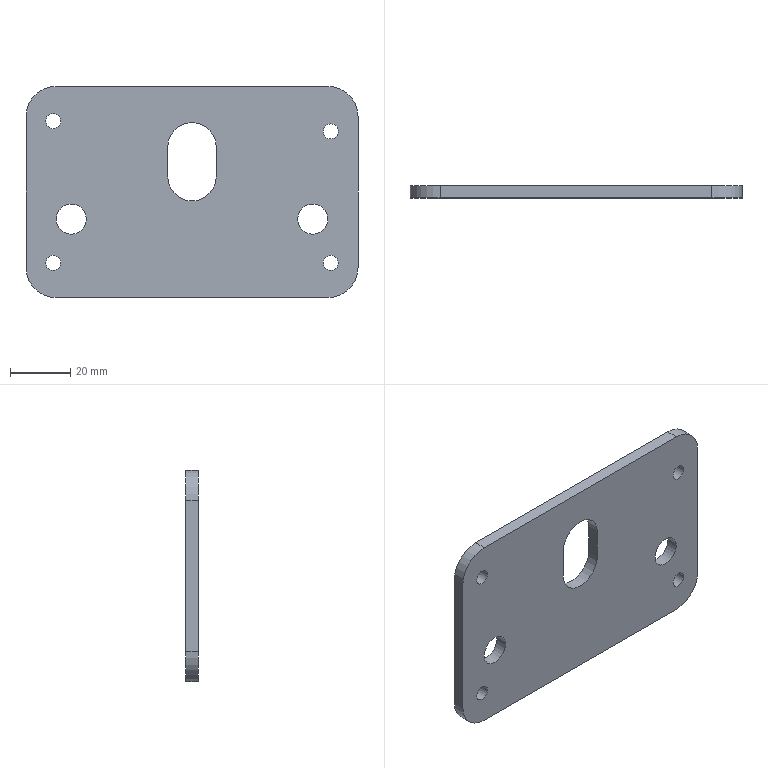Part | STEP file | 10 | 1 solid | 20 faces | box 110 x 4 x 70 mm | volume 28070 mm3 | cylinder 12 | plane 8 | commonest cylinder face diameters 5 x4 20 x4 10 x2 16 x2